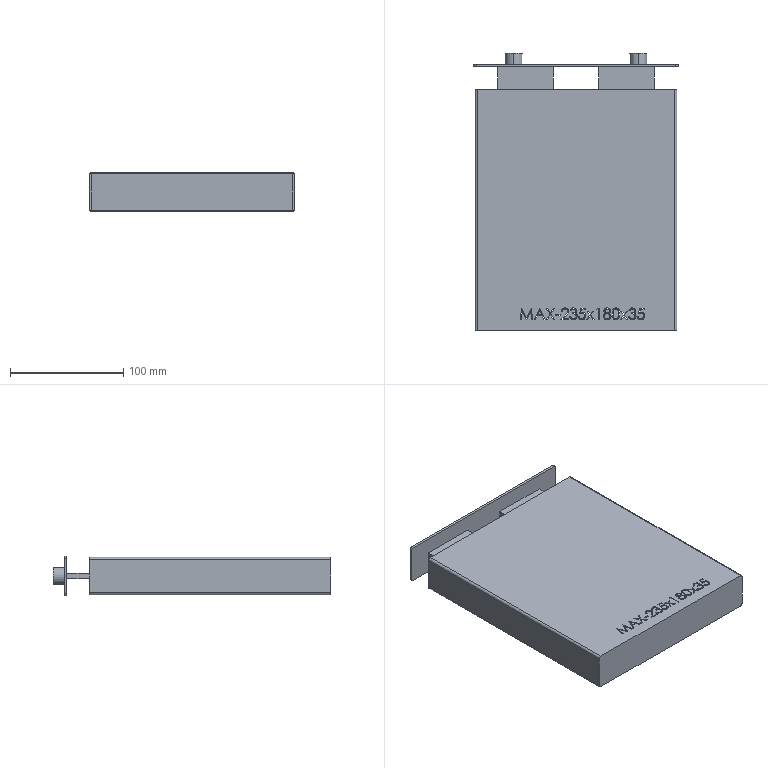Part | STEP file | MAX-Cell | 5 solids | 212 faces | box 180 x 245 x 35 mm | volume 1267148 mm3 | plane 124 | spline 76 | cylinder 12 | commonest cylinder face diameters 4 x8 15 x4